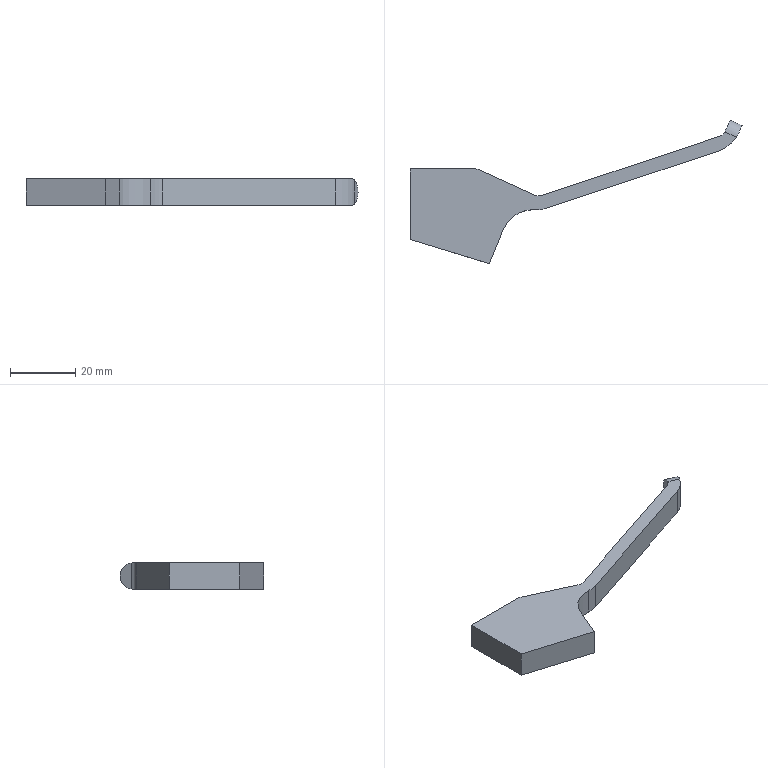Part | STEP file | Dual Brake Lever Arm | 1 solid | 19 faces | box 101.987 x 44.103 x 8 mm | volume 8520 mm3 | plane 11 | cylinder 8 | commonest cylinder face diameters 6 x3 20 x3 8 x2